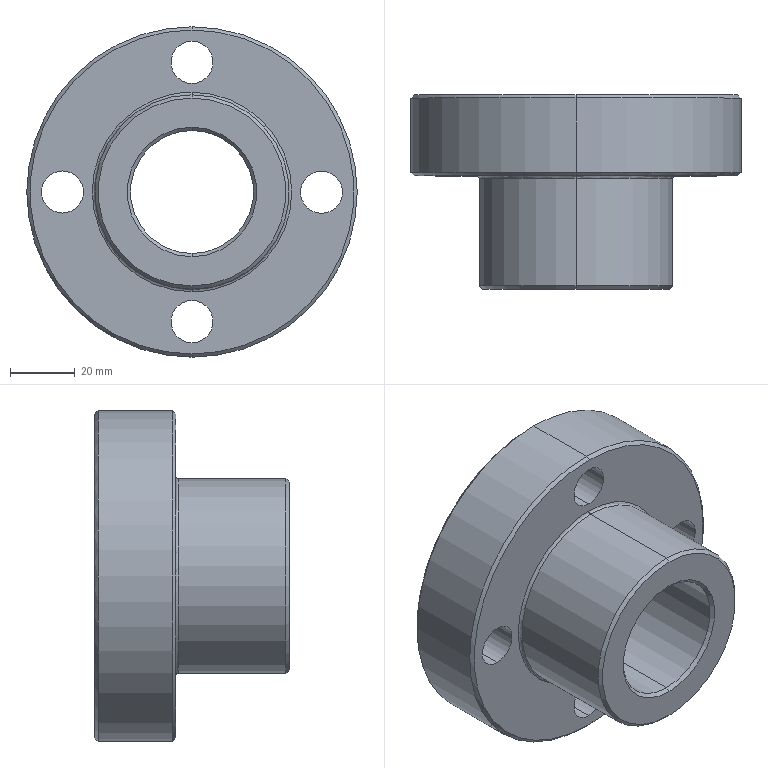Part | SolidWorks | features BaseBody 1 | 1 solid | 29 faces | box 102 x 60 x 102 mm | volume 221417 mm3 | cylinder 14 | cone 10 | plane 3 | spline 2 | commonest cylinder face diameters 13 x8 38 x2 60 x2 102 x2